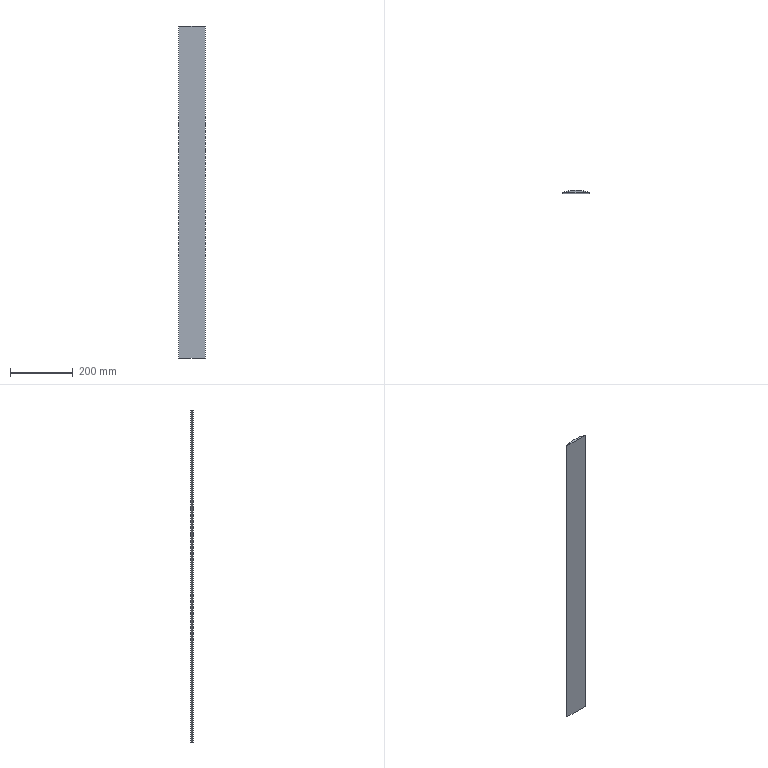Part | SolidWorks | features BaseBody 1 | 1 solid | 24 faces | box 84 x 8.038 x 1060 mm | volume 538813 mm3 | cylinder 19 | plane 5 | commonest cylinder face diameters 0.6 x8 303 x5 0.8 x4 4 x2
STEP:
#1=CARTESIAN_POINT('',(42.,-0.03816,1060.));
#2=VERTEX_POINT('',#1);
#3=CARTESIAN_POINT('',(42.,-0.03816,0.));
#4=VERTEX_POINT('',#3);
#5=CARTESIAN_POINT('',(42.,-0.03816,1060.));
#6=DIRECTION('',(0.,0.,-1.));
#7=VECTOR('',#6,1000.);
#8=LINE('',#5,#7);
#9=EDGE_CURVE('',#2,#4,#8,.T.);
#10=ORIENTED_EDGE('',*,*,#9,.F.);
#11=CARTESIAN_POINT('',(-42.,-0.03816,1060.));
#12=VERTEX_POINT('',#11);
#13=CARTESIAN_POINT('',(-40.,-0.03816,1060.));
#14=DIRECTION('',(1.,0.,0.));
#15=VECTOR('',#14,1000.);
#16=LINE('',#13,#15);
#17=EDGE_CURVE('',#12,#2,#16,.T.);
#18=ORIENTED_EDGE('',*,*,#17,.F.);
#19=CARTESIAN_POINT('',(-42.,-0.03816,0.));
#20=VERTEX_POINT('',#19);
#21=CARTESIAN_POINT('',(-42.,-0.03816,1060.));
#22=DIRECTION('',(0.,0.,1.));
#23=VECTOR('',#22,1000.);
#24=LINE('',#21,#23);
#25=EDGE_CURVE('',#20,#12,#24,.T.);
#26=ORIENTED_EDGE('',*,*,#25,.F.);
#27=CARTESIAN_POINT('',(-40.,-0.03816,0.));
#28=DIRECTION('',(-1.,0.,0.));
#29=VECTOR('',#28,1000.);
#30=LINE('',#27,#29);
#31=EDGE_CURVE('',#4,#20,#30,.T.);
#32=ORIENTED_EDGE('',*,*,#31,.F.);
#33=EDGE_LOOP('',(#10,#18,#26,#32));
#34=FACE_OUTER_BOUND('',#33,.T.);
#35=CARTESIAN_POINT('',(-40.,-0.03816,1060.));
#36=DIRECTION('',(0.,1.,0.));
#37=DIRECTION('',(-1.,0.,0.));
#38=AXIS2_PLACEMENT_3D('',#35,#36,#37);
#39=PLANE('',#38);
#40=ADVANCED_FACE('',(#34),#39,.F.);
#41=CARTESIAN_POINT('',(-40.535,2.477,0.));
#42=VERTEX_POINT('',#41);
#43=CARTESIAN_POINT('',(-42.,0.5495,0.));
#44=VERTEX_POINT('',#43);
#45=CARTESIAN_POINT('',(-40.,0.5495,0.));
#46=DIRECTION('',(0.,0.,1.));
#47=DIRECTION('',(-1.,0.,0.));
#48=AXIS2_PLACEMENT_3D('',#45,#46,#47);
#49=CIRCLE('',#48,2.);
#50=EDGE_CURVE('',#42,#44,#49,.T.);
#51=ORIENTED_EDGE('',*,*,#50,.F.);
#52=CARTESIAN_POINT('',(-25.125,5.902,0.));
#53=VERTEX_POINT('',#52);
#54=CARTESIAN_POINT('',(0.,-143.5,0.));
#55=DIRECTION('',(0.,0.,1.));
#56=DIRECTION('',(-1.,0.,0.));
#57=AXIS2_PLACEMENT_3D('',#54,#55,#56);
#58=CIRCLE('',#57,151.5);
#59=EDGE_CURVE('',#53,#42,#58,.T.);
#60=ORIENTED_EDGE('',*,*,#59,.F.);
#61=CARTESIAN_POINT('',(-24.828,5.778,0.));
#62=VERTEX_POINT('',#61);
#63=CARTESIAN_POINT('',(-25.075,5.606,0.));
#64=DIRECTION('',(0.,0.,1.));
#65=DIRECTION('',(-1.,0.,0.));
#66=AXIS2_PLACEMENT_3D('',#63,#64,#65);
#67=CIRCLE('',#66,0.3);
#68=EDGE_CURVE('',#62,#53,#67,.T.);
#69=ORIENTED_EDGE('',*,*,#68,.F.);
#70=CARTESIAN_POINT('',(-24.116,5.894,0.));
#71=VERTEX_POINT('',#70);
#72=CARTESIAN_POINT('',(-24.5,6.006,0.));
#73=DIRECTION('',(0.,0.,1.));
#74=DIRECTION('',(-1.,0.,0.));
#75=AXIS2_PLACEMENT_3D('',#72,#73,#74);
#76=CIRCLE('',#75,0.4);
#77=EDGE_CURVE('',#62,#71,#76,.T.);
#78=ORIENTED_EDGE('',*,*,#77,.T.);
#79=CARTESIAN_POINT('',(-23.875,6.107,0.));
#80=VERTEX_POINT('',#79);
#81=CARTESIAN_POINT('',(-23.828,5.811,0.));
#82=DIRECTION('',(0.,0.,1.));
#83=DIRECTION('',(-1.,0.,0.));
#84=AXIS2_PLACEMENT_3D('',#81,#82,#83);
#85=CIRCLE('',#84,0.3);
#86=EDGE_CURVE('',#80,#71,#85,.T.);
#87=ORIENTED_EDGE('',*,*,#86,.F.);
#88=CARTESIAN_POINT('',(-23.626,6.147,0.));
#89=VERTEX_POINT('',#88);
#90=CARTESIAN_POINT('',(0.,-143.5,0.));
#91=DIRECTION('',(0.,0.,1.));
#92=DIRECTION('',(-1.,0.,0.));
#93=AXIS2_PLACEMENT_3D('',#90,#91,#92);
#94=CIRCLE('',#93,151.5);
#95=EDGE_CURVE('',#89,#80,#94,.T.);
#96=ORIENTED_EDGE('',*,*,#95,.F.);
#97=CARTESIAN_POINT('',(-23.331,6.019,0.));
#98=VERTEX_POINT('',#97);
#99=CARTESIAN_POINT('',(-23.579,5.85,0.));
#100=DIRECTION('',(0.,0.,1.));
#101=DIRECTION('',(-1.,0.,0.));
#102=AXIS2_PLACEMENT_3D('',#99,#100,#101);
#103=CIRCLE('',#102,0.3);
#104=EDGE_CURVE('',#98,#89,#103,.T.);
#105=ORIENTED_EDGE('',*,*,#104,.F.);
#106=CARTESIAN_POINT('',(-22.617,6.129,0.));
#107=VERTEX_POINT('',#106);
#108=CARTESIAN_POINT('',(-23.,6.244,0.));
#109=DIRECTION('',(0.,0.,1.));
#110=DIRECTION('',(-1.,0.,0.));
#111=AXIS2_PLACEMENT_3D('',#108,#109,#110);
#112=CIRCLE('',#111,0.4);
#113=EDGE_CURVE('',#98,#107,#112,.T.);
#114=ORIENTED_EDGE('',*,*,#113,.T.);
#115=CARTESIAN_POINT('',(-22.374,6.339,0.));
#116=VERTEX_POINT('',#115);
#117=CARTESIAN_POINT('',(-22.33,6.042,0.));
#118=DIRECTION('',(0.,0.,1.));
#119=DIRECTION('',(-1.,0.,0.));
#120=AXIS2_PLACEMENT_3D('',#117,#118,#119);
#121=CIRCLE('',#120,0.3);
#122=EDGE_CURVE('',#116,#107,#121,.T.);
#123=ORIENTED_EDGE('',*,*,#122,.F.);
#124=CARTESIAN_POINT('',(22.374,6.339,0.));
#125=VERTEX_POINT('',#124);
#126=CARTESIAN_POINT('',(0.,-143.5,0.));
#127=DIRECTION('',(0.,0.,1.));
#128=DIRECTION('',(-1.,0.,0.));
#129=AXIS2_PLACEMENT_3D('',#126,#127,#128);
#130=CIRCLE('',#129,151.5);
#131=EDGE_CURVE('',#125,#116,#130,.T.);
#132=ORIENTED_EDGE('',*,*,#131,.F.);
#133=CARTESIAN_POINT('',(22.617,6.129,0.));
#134=VERTEX_POINT('',#133);
#135=CARTESIAN_POINT('',(22.33,6.042,0.));
#136=DIRECTION('',(0.,0.,1.));
#137=DIRECTION('',(-1.,0.,0.));
#138=AXIS2_PLACEMENT_3D('',#135,#136,#137);
#139=CIRCLE('',#138,0.3);
#140=EDGE_CURVE('',#134,#125,#139,.T.);
#141=ORIENTED_EDGE('',*,*,#140,.F.);
#142=CARTESIAN_POINT('',(23.331,6.019,0.));
#143=VERTEX_POINT('',#142);
#144=CARTESIAN_POINT('',(23.,6.244,0.));
#145=DIRECTION('',(0.,0.,1.));
#146=DIRECTION('',(-1.,0.,0.));
#147=AXIS2_PLACEMENT_3D('',#144,#145,#146);
#148=CIRCLE('',#147,0.4);
#149=EDGE_CURVE('',#134,#143,#148,.T.);
#150=ORIENTED_EDGE('',*,*,#149,.T.);
#151=CARTESIAN_POINT('',(23.626,6.147,0.));
#152=VERTEX_POINT('',#151);
#153=CARTESIAN_POINT('',(23.579,5.85,0.));
#154=DIRECTION('',(0.,0.,1.));
#155=DIRECTION('',(-1.,0.,0.));
#156=AXIS2_PLACEMENT_3D('',#153,#154,#155);
#157=CIRCLE('',#156,0.3);
#158=EDGE_CURVE('',#152,#143,#157,.T.);
#159=ORIENTED_EDGE('',*,*,#158,.F.);
#160=CARTESIAN_POINT('',(23.875,6.107,0.));
#161=VERTEX_POINT('',#160);
#162=CARTESIAN_POINT('',(0.,-143.5,0.));
#163=DIRECTION('',(0.,0.,1.));
#164=DIRECTION('',(-1.,0.,0.));
#165=AXIS2_PLACEMENT_3D('',#162,#163,#164);
#166=CIRCLE('',#165,151.5);
#167=EDGE_CURVE('',#161,#152,#166,.T.);
#168=ORIENTED_EDGE('',*,*,#167,.F.);
#169=CARTESIAN_POINT('',(24.116,5.894,0.));
#170=VERTEX_POINT('',#169);
#171=CARTESIAN_POINT('',(23.828,5.811,0.));
#172=DIRECTION('',(0.,0.,1.));
#173=DIRECTION('',(-1.,0.,0.));
#174=AXIS2_PLACEMENT_3D('',#171,#172,#173);
#175=CIRCLE('',#174,0.3);
#176=EDGE_CURVE('',#170,#161,#175,.T.);
#177=ORIENTED_EDGE('',*,*,#176,.F.);
#178=CARTESIAN_POINT('',(24.828,5.778,0.));
#179=VERTEX_POINT('',#178);
#180=CARTESIAN_POINT('',(24.5,6.006,0.));
#181=DIRECTION('',(0.,0.,1.));
#182=DIRECTION('',(-1.,0.,0.));
#183=AXIS2_PLACEMENT_3D('',#180,#181,#182);
#184=CIRCLE('',#183,0.4);
#185=EDGE_CURVE('',#170,#179,#184,.T.);
#186=ORIENTED_EDGE('',*,*,#185,.T.);
#187=CARTESIAN_POINT('',(25.125,5.902,0.));
#188=VERTEX_POINT('',#187);
#189=CARTESIAN_POINT('',(25.075,5.606,0.));
#190=DIRECTION('',(0.,0.,1.));
#191=DIRECTION('',(-1.,0.,0.));
#192=AXIS2_PLACEMENT_3D('',#189,#190,#191);
#193=CIRCLE('',#192,0.3);
#194=EDGE_CURVE('',#188,#179,#193,.T.);
#195=ORIENTED_EDGE('',*,*,#194,.F.);
#196=CARTESIAN_POINT('',(40.535,2.477,0.));
#197=VERTEX_POINT('',#196);
#198=CARTESIAN_POINT('',(0.,-143.5,0.));
#199=DIRECTION('',(0.,0.,1.));
#200=DIRECTION('',(-1.,0.,0.));
#201=AXIS2_PLACEMENT_3D('',#198,#199,#200);
#202=CIRCLE('',#201,151.5);
#203=EDGE_CURVE('',#197,#188,#202,.T.);
#204=ORIENTED_EDGE('',*,*,#203,.F.);
#205=CARTESIAN_POINT('',(42.,0.5495,0.));
#206=VERTEX_POINT('',#205);
#207=CARTESIAN_POINT('',(40.,0.5495,0.));
#208=DIRECTION('',(0.,0.,1.));
#209=DIRECTION('',(-1.,0.,0.));
#210=AXIS2_PLACEMENT_3D('',#207,#208,#209);
#211=CIRCLE('',#210,2.);
#212=EDGE_CURVE('',#206,#197,#211,.T.);
#213=ORIENTED_EDGE('',*,*,#212,.F.);
#214=CARTESIAN_POINT('',(42.,-143.5,0.));
#215=DIRECTION('',(0.,1.,0.));
#216=VECTOR('',#215,1000.);
#217=LINE('',#214,#216);
#218=EDGE_CURVE('',#4,#206,#217,.T.);
#219=ORIENTED_EDGE('',*,*,#218,.F.);
#220=ORIENTED_EDGE('',*,*,#31,.T.);
#221=CARTESIAN_POINT('',(-42.,-143.5,0.));
#222=DIRECTION('',(0.,-1.,0.));
#223=VECTOR('',#222,1000.);
#224=LINE('',#221,#223);
#225=EDGE_CURVE('',#44,#20,#224,.T.);
#226=ORIENTED_EDGE('',*,*,#225,.F.);
#227=EDGE_LOOP('',(#51,#60,#69,#78,#87,#96,#105,#114,#123,#132,#141,#150,#159,#168,#177,#186,#195,#204,#213,#219,#220,#226));
#228=FACE_OUTER_BOUND('',#227,.T.);
#229=CARTESIAN_POINT('',(0.,-143.5,0.));
#230=DIRECTION('',(0.,0.,1.));
#231=DIRECTION('',(1.,0.,0.));
#232=AXIS2_PLACEMENT_3D('',#229,#230,#231);
#233=PLANE('',#232);
#234=ADVANCED_FACE('',(#228),#233,.F.);
#235=CARTESIAN_POINT('',(42.,0.5495,1060.));
#236=VERTEX_POINT('',#235);
#237=CARTESIAN_POINT('',(42.,0.5495,1060.));
#238=DIRECTION('',(0.,0.,-1.));
#239=VECTOR('',#238,1000.);
#240=LINE('',#237,#239);
#241=EDGE_CURVE('',#236,#206,#240,.T.);
#242=ORIENTED_EDGE('',*,*,#241,.F.);
#243=CARTESIAN_POINT('',(42.,2.062,1060.));
#244=DIRECTION('',(0.,1.,0.));
#245=VECTOR('',#244,1000.);
#246=LINE('',#243,#245);
#247=EDGE_CURVE('',#2,#236,#246,.T.);
#248=ORIENTED_EDGE('',*,*,#247,.F.);
#249=ORIENTED_EDGE('',*,*,#9,.T.);
#250=ORIENTED_EDGE('',*,*,#218,.T.);
#251=EDGE_LOOP('',(#242,#248,#249,#250));
#252=FACE_OUTER_BOUND('',#251,.T.);
#253=CARTESIAN_POINT('',(42.,2.062,1060.));
#254=DIRECTION('',(-1.,0.,0.));
#255=DIRECTION('',(0.,0.,1.));
#256=AXIS2_PLACEMENT_3D('',#253,#254,#255);
#257=PLANE('',#256);
#258=ADVANCED_FACE('',(#252),#257,.F.);
#259=CARTESIAN_POINT('',(-24.116,5.894,1060.));
#260=VERTEX_POINT('',#259);
#261=CARTESIAN_POINT('',(-24.828,5.778,1060.));
#262=VERTEX_POINT('',#261);
#263=CARTESIAN_POINT('',(-24.5,6.006,1060.));
#264=DIRECTION('',(0.,0.,-1.));
#265=DIRECTION('',(-1.,0.,0.));
#266=AXIS2_PLACEMENT_3D('',#263,#264,#265);
#267=CIRCLE('',#266,0.4);
#268=EDGE_CURVE('',#260,#262,#267,.T.);
#269=ORIENTED_EDGE('',*,*,#268,.T.);
#270=CARTESIAN_POINT('',(-25.125,5.902,1060.));
#271=VERTEX_POINT('',#270);
#272=CARTESIAN_POINT('',(-25.075,5.606,1060.));
#273=DIRECTION('',(0.,0.,-1.));
#274=DIRECTION('',(-1.,0.,0.));
#275=AXIS2_PLACEMENT_3D('',#272,#273,#274);
#276=CIRCLE('',#275,0.3);
#277=EDGE_CURVE('',#271,#262,#276,.T.);
#278=ORIENTED_EDGE('',*,*,#277,.F.);
#279=CARTESIAN_POINT('',(-40.535,2.477,1060.));
#280=VERTEX_POINT('',#279);
#281=CARTESIAN_POINT('',(0.,-143.5,1060.));
#282=DIRECTION('',(0.,0.,1.));
#283=DIRECTION('',(-1.,0.,0.));
#284=AXIS2_PLACEMENT_3D('',#281,#282,#283);
#285=CIRCLE('',#284,151.5);
#286=EDGE_CURVE('',#271,#280,#285,.T.);
#287=ORIENTED_EDGE('',*,*,#286,.T.);
#288=CARTESIAN_POINT('',(-42.,0.5495,1060.));
#289=VERTEX_POINT('',#288);
#290=CARTESIAN_POINT('',(-40.,0.5495,1060.));
#291=DIRECTION('',(0.,0.,1.));
#292=DIRECTION('',(-1.,0.,0.));
#293=AXIS2_PLACEMENT_3D('',#290,#291,#292);
#294=CIRCLE('',#293,2.);
#295=EDGE_CURVE('',#280,#289,#294,.T.);
#296=ORIENTED_EDGE('',*,*,#295,.T.);
#297=CARTESIAN_POINT('',(-42.,-143.5,1060.));
#298=DIRECTION('',(0.,-1.,0.));
#299=VECTOR('',#298,1000.);
#300=LINE('',#297,#299);
#301=EDGE_CURVE('',#289,#12,#300,.T.);
#302=ORIENTED_EDGE('',*,*,#301,.T.);
#303=ORIENTED_EDGE('',*,*,#17,.T.);
#304=ORIENTED_EDGE('',*,*,#247,.T.);
#305=CARTESIAN_POINT('',(40.535,2.477,1060.));
#306=VERTEX_POINT('',#305);
#307=CARTESIAN_POINT('',(40.,0.5495,1060.));
#308=DIRECTION('',(0.,0.,1.));
#309=DIRECTION('',(-1.,0.,0.));
#310=AXIS2_PLACEMENT_3D('',#307,#308,#309);
#311=CIRCLE('',#310,2.);
#312=EDGE_CURVE('',#236,#306,#311,.T.);
#313=ORIENTED_EDGE('',*,*,#312,.T.);
#314=CARTESIAN_POINT('',(25.125,5.902,1060.));
#315=VERTEX_POINT('',#314);
#316=CARTESIAN_POINT('',(0.,-143.5,1060.));
#317=DIRECTION('',(0.,0.,1.));
#318=DIRECTION('',(-1.,0.,0.));
#319=AXIS2_PLACEMENT_3D('',#316,#317,#318);
#320=CIRCLE('',#319,151.5);
#321=EDGE_CURVE('',#306,#315,#320,.T.);
#322=ORIENTED_EDGE('',*,*,#321,.T.);
#323=CARTESIAN_POINT('',(24.828,5.778,1060.));
#324=VERTEX_POINT('',#323);
#325=CARTESIAN_POINT('',(25.075,5.606,1060.));
#326=DIRECTION('',(0.,0.,-1.));
#327=DIRECTION('',(-1.,0.,0.));
#328=AXIS2_PLACEMENT_3D('',#325,#326,#327);
#329=CIRCLE('',#328,0.3);
#330=EDGE_CURVE('',#324,#315,#329,.T.);
#331=ORIENTED_EDGE('',*,*,#330,.F.);
#332=CARTESIAN_POINT('',(24.116,5.894,1060.));
#333=VERTEX_POINT('',#332);
#334=CARTESIAN_POINT('',(24.5,6.006,1060.));
#335=DIRECTION('',(0.,0.,-1.));
#336=DIRECTION('',(-1.,0.,0.));
#337=AXIS2_PLACEMENT_3D('',#334,#335,#336);
#338=CIRCLE('',#337,0.4);
#339=EDGE_CURVE('',#324,#333,#338,.T.);
#340=ORIENTED_EDGE('',*,*,#339,.T.);
#341=CARTESIAN_POINT('',(23.875,6.107,1060.));
#342=VERTEX_POINT('',#341);
#343=CARTESIAN_POINT('',(23.828,5.811,1060.));
#344=DIRECTION('',(0.,0.,-1.));
#345=DIRECTION('',(-1.,0.,0.));
#346=AXIS2_PLACEMENT_3D('',#343,#344,#345);
#347=CIRCLE('',#346,0.3);
#348=EDGE_CURVE('',#342,#333,#347,.T.);
#349=ORIENTED_EDGE('',*,*,#348,.F.);
#350=CARTESIAN_POINT('',(23.626,6.147,1060.));
#351=VERTEX_POINT('',#350);
#352=CARTESIAN_POINT('',(0.,-143.5,1060.));
#353=DIRECTION('',(0.,0.,-1.));
#354=DIRECTION('',(-1.,0.,0.));
#355=AXIS2_PLACEMENT_3D('',#352,#353,#354);
#356=CIRCLE('',#355,151.5);
#357=EDGE_CURVE('',#351,#342,#356,.T.);
#358=ORIENTED_EDGE('',*,*,#357,.F.);
#359=CARTESIAN_POINT('',(23.331,6.019,1060.));
#360=VERTEX_POINT('',#359);
#361=CARTESIAN_POINT('',(23.579,5.85,1060.));
#362=DIRECTION('',(0.,0.,-1.));
#363=DIRECTION('',(-1.,0.,0.));
#364=AXIS2_PLACEMENT_3D('',#361,#362,#363);
#365=CIRCLE('',#364,0.3);
#366=EDGE_CURVE('',#360,#351,#365,.T.);
#367=ORIENTED_EDGE('',*,*,#366,.F.);
#368=CARTESIAN_POINT('',(22.617,6.129,1060.));
#369=VERTEX_POINT('',#368);
#370=CARTESIAN_POINT('',(23.,6.244,1060.));
#371=DIRECTION('',(0.,0.,-1.));
#372=DIRECTION('',(-1.,0.,0.));
#373=AXIS2_PLACEMENT_3D('',#370,#371,#372);
#374=CIRCLE('',#373,0.4);
#375=EDGE_CURVE('',#360,#369,#374,.T.);
#376=ORIENTED_EDGE('',*,*,#375,.T.);
#377=CARTESIAN_POINT('',(22.374,6.339,1060.));
#378=VERTEX_POINT('',#377);
#379=CARTESIAN_POINT('',(22.33,6.042,1060.));
#380=DIRECTION('',(0.,0.,-1.));
#381=DIRECTION('',(-1.,0.,0.));
#382=AXIS2_PLACEMENT_3D('',#379,#380,#381);
#383=CIRCLE('',#382,0.3);
#384=EDGE_CURVE('',#378,#369,#383,.T.);
#385=ORIENTED_EDGE('',*,*,#384,.F.);
#386=CARTESIAN_POINT('',(-22.374,6.339,1060.));
#387=VERTEX_POINT('',#386);
#388=CARTESIAN_POINT('',(0.,-143.5,1060.));
#389=DIRECTION('',(0.,0.,1.));
#390=DIRECTION('',(-1.,0.,0.));
#391=AXIS2_PLACEMENT_3D('',#388,#389,#390);
#392=CIRCLE('',#391,151.5);
#393=EDGE_CURVE('',#378,#387,#392,.T.);
#394=ORIENTED_EDGE('',*,*,#393,.T.);
#395=CARTESIAN_POINT('',(-22.617,6.129,1060.));
#396=VERTEX_POINT('',#395);
#397=CARTESIAN_POINT('',(-22.33,6.042,1060.));
#398=DIRECTION('',(0.,0.,-1.));
#399=DIRECTION('',(-1.,0.,0.));
#400=AXIS2_PLACEMENT_3D('',#397,#398,#399);
#401=CIRCLE('',#400,0.3);
#402=EDGE_CURVE('',#396,#387,#401,.T.);
#403=ORIENTED_EDGE('',*,*,#402,.F.);
#404=CARTESIAN_POINT('',(-23.331,6.019,1060.));
#405=VERTEX_POINT('',#404);
#406=CARTESIAN_POINT('',(-23.,6.244,1060.));
#407=DIRECTION('',(0.,0.,-1.));
#408=DIRECTION('',(-1.,0.,0.));
#409=AXIS2_PLACEMENT_3D('',#406,#407,#408);
#410=CIRCLE('',#409,0.4);
#411=EDGE_CURVE('',#396,#405,#410,.T.);
#412=ORIENTED_EDGE('',*,*,#411,.T.);
#413=CARTESIAN_POINT('',(-23.626,6.147,1060.));
#414=VERTEX_POINT('',#413);
#415=CARTESIAN_POINT('',(-23.579,5.85,1060.));
#416=DIRECTION('',(0.,0.,-1.));
#417=DIRECTION('',(-1.,0.,0.));
#418=AXIS2_PLACEMENT_3D('',#415,#416,#417);
#419=CIRCLE('',#418,0.3);
#420=EDGE_CURVE('',#414,#405,#419,.T.);
#421=ORIENTED_EDGE('',*,*,#420,.F.);
#422=CARTESIAN_POINT('',(-23.875,6.107,1060.));
#423=VERTEX_POINT('',#422);
#424=CARTESIAN_POINT('',(0.,-143.5,1060.));
#425=DIRECTION('',(0.,0.,-1.));
#426=DIRECTION('',(-1.,0.,0.));
#427=AXIS2_PLACEMENT_3D('',#424,#425,#426);
#428=CIRCLE('',#427,151.5);
#429=EDGE_CURVE('',#423,#414,#428,.T.);
#430=ORIENTED_EDGE('',*,*,#429,.F.);
#431=CARTESIAN_POINT('',(-23.828,5.811,1060.));
#432=DIRECTION('',(0.,0.,-1.));
#433=DIRECTION('',(-1.,0.,0.));
#434=AXIS2_PLACEMENT_3D('',#431,#432,#433);
#435=CIRCLE('',#434,0.3);
#436=EDGE_CURVE('',#260,#423,#435,.T.);
#437=ORIENTED_EDGE('',*,*,#436,.F.);
#438=EDGE_LOOP('',(#269,#278,#287,#296,#302,#303,#304,#313,#322,#331,#340,#349,#358,#367,#376,#385,#394,#403,#412,#421,#430,#437));
#439=FACE_OUTER_BOUND('',#438,.T.);
#440=CARTESIAN_POINT('',(0.,-143.5,1060.));
#441=DIRECTION('',(0.,0.,1.));
#442=DIRECTION('',(1.,0.,0.));
#443=AXIS2_PLACEMENT_3D('',#440,#441,#442);
#444=PLANE('',#443);
#445=ADVANCED_FACE('',(#439),#444,.T.);
#446=CARTESIAN_POINT('',(-42.,0.5495,1060.));
#447=DIRECTION('',(0.,0.,1.));
#448=VECTOR('',#447,1000.);
#449=LINE('',#446,#448);
#450=EDGE_CURVE('',#44,#289,#449,.T.);
#451=ORIENTED_EDGE('',*,*,#450,.F.);
#452=ORIENTED_EDGE('',*,*,#225,.T.);
#453=ORIENTED_EDGE('',*,*,#25,.T.);
#454=ORIENTED_EDGE('',*,*,#301,.F.);
#455=EDGE_LOOP('',(#451,#452,#453,#454));
#456=FACE_OUTER_BOUND('',#455,.T.);
#457=CARTESIAN_POINT('',(-42.,2.062,1060.));
#458=DIRECTION('',(1.,0.,0.));
#459=DIRECTION('',(0.,0.,-1.));
#460=AXIS2_PLACEMENT_3D('',#457,#458,#459);
#461=PLANE('',#460);
#462=ADVANCED_FACE('',(#456),#461,.F.);
#463=ORIENTED_EDGE('',*,*,#50,.T.);
#464=ORIENTED_EDGE('',*,*,#450,.T.);
#465=ORIENTED_EDGE('',*,*,#295,.F.);
#466=CARTESIAN_POINT('',(-40.535,2.477,1060.));
#467=DIRECTION('',(0.,0.,-1.));
#468=VECTOR('',#467,1000.);
#469=LINE('',#466,#468);
#470=EDGE_CURVE('',#280,#42,#469,.T.);
#471=ORIENTED_EDGE('',*,*,#470,.T.);
#472=EDGE_LOOP('',(#463,#464,#465,#471));
#473=FACE_OUTER_BOUND('',#472,.T.);
#474=CARTESIAN_POINT('',(-40.,0.5495,1060.));
#475=DIRECTION('',(0.,0.,-1.));
#476=DIRECTION('',(-1.,0.,0.));
#477=AXIS2_PLACEMENT_3D('',#474,#475,#476);
#478=CYLINDRICAL_SURFACE('',#477,2.);
#479=ADVANCED_FACE('',(#473),#478,.T.);
#480=ORIENTED_EDGE('',*,*,#286,.F.);
#481=CARTESIAN_POINT('',(-25.125,5.902,1060.));
#482=DIRECTION('',(0.,0.,-1.));
#483=VECTOR('',#482,1000.);
#484=LINE('',#481,#483);
#485=EDGE_CURVE('',#271,#53,#484,.T.);
#486=ORIENTED_EDGE('',*,*,#485,.T.);
#487=ORIENTED_EDGE('',*,*,#59,.T.);
#488=ORIENTED_EDGE('',*,*,#470,.F.);
#489=EDGE_LOOP('',(#480,#486,#487,#488));
#490=FACE_OUTER_BOUND('',#489,.T.);
#491=CARTESIAN_POINT('',(0.,-143.5,1060.));
#492=DIRECTION('',(0.,0.,-1.));
#493=DIRECTION('',(-1.,0.,0.));
#494=AXIS2_PLACEMENT_3D('',#491,#492,#493);
#495=CYLINDRICAL_SURFACE('',#494,151.5);
#496=ADVANCED_FACE('',(#490),#495,.T.);
#497=ORIENTED_EDGE('',*,*,#393,.F.);
#498=CARTESIAN_POINT('',(22.374,6.339,1060.));
#499=DIRECTION('',(0.,0.,-1.));
#500=VECTOR('',#499,1000.);
#501=LINE('',#498,#500);
#502=EDGE_CURVE('',#378,#125,#501,.T.);
#503=ORIENTED_EDGE('',*,*,#502,.T.);
#504=ORIENTED_EDGE('',*,*,#131,.T.);
#505=CARTESIAN_POINT('',(-22.374,6.339,1060.));
#506=DIRECTION('',(0.,0.,1.));
#507=VECTOR('',#506,1000.);
#508=LINE('',#505,#507);
#509=EDGE_CURVE('',#116,#387,#508,.T.);
#510=ORIENTED_EDGE('',*,*,#509,.T.);
#511=EDGE_LOOP('',(#497,#503,#504,#510));
#512=FACE_OUTER_BOUND('',#511,.T.);
#513=CARTESIAN_POINT('',(0.,-143.5,1060.));
#514=DIRECTION('',(0.,0.,-1.));
#515=DIRECTION('',(-1.,0.,0.));
#516=AXIS2_PLACEMENT_3D('',#513,#514,#515);
#517=CYLINDRICAL_SURFACE('',#516,151.5);
#518=ADVANCED_FACE('',(#512),#517,.T.);
#519=ORIENTED_EDGE('',*,*,#203,.T.);
#520=CARTESIAN_POINT('',(25.125,5.902,1060.));
#521=DIRECTION('',(0.,0.,1.));
#522=VECTOR('',#521,1000.);
#523=LINE('',#520,#522);
#524=EDGE_CURVE('',#188,#315,#523,.T.);
#525=ORIENTED_EDGE('',*,*,#524,.T.);
#526=ORIENTED_EDGE('',*,*,#321,.F.);
#527=CARTESIAN_POINT('',(40.535,2.477,1060.));
#528=DIRECTION('',(0.,0.,-1.));
#529=VECTOR('',#528,1000.);
#530=LINE('',#527,#529);
#531=EDGE_CURVE('',#306,#197,#530,.T.);
#532=ORIENTED_EDGE('',*,*,#531,.T.);
#533=EDGE_LOOP('',(#519,#525,#526,#532));
#534=FACE_OUTER_BOUND('',#533,.T.);
#535=CARTESIAN_POINT('',(0.,-143.5,1060.));
#536=DIRECTION('',(0.,0.,-1.));
#537=DIRECTION('',(-1.,0.,0.));
#538=AXIS2_PLACEMENT_3D('',#535,#536,#537);
#539=CYLINDRICAL_SURFACE('',#538,151.5);
#540=ADVANCED_FACE('',(#534),#539,.T.);
#541=ORIENTED_EDGE('',*,*,#212,.T.);
#542=ORIENTED_EDGE('',*,*,#531,.F.);
#543=ORIENTED_EDGE('',*,*,#312,.F.);
#544=ORIENTED_EDGE('',*,*,#241,.T.);
#545=EDGE_LOOP('',(#541,#542,#543,#544));
#546=FACE_OUTER_BOUND('',#545,.T.);
#547=CARTESIAN_POINT('',(40.,0.5495,1060.));
#548=DIRECTION('',(0.,0.,-1.));
#549=DIRECTION('',(-1.,0.,0.));
#550=AXIS2_PLACEMENT_3D('',#547,#548,#549);
#551=CYLINDRICAL_SURFACE('',#550,2.);
#552=ADVANCED_FACE('',(#546),#551,.T.);
#553=ORIENTED_EDGE('',*,*,#277,.T.);
#554=CARTESIAN_POINT('',(-24.828,5.778,1060.));
#555=DIRECTION('',(0.,0.,-1.));
#556=VECTOR('',#555,1000.);
#557=LINE('',#554,#556);
#558=EDGE_CURVE('',#262,#62,#557,.T.);
#559=ORIENTED_EDGE('',*,*,#558,.T.);
#560=ORIENTED_EDGE('',*,*,#68,.T.);
#561=ORIENTED_EDGE('',*,*,#485,.F.);
#562=EDGE_LOOP('',(#553,#559,#560,#561));
#563=FACE_OUTER_BOUND('',#562,.T.);
#564=CARTESIAN_POINT('',(-25.075,5.606,1060.));
#565=DIRECTION('',(0.,0.,-1.));
#566=DIRECTION('',(-1.,0.,0.));
#567=AXIS2_PLACEMENT_3D('',#564,#565,#566);
#568=CYLINDRICAL_SURFACE('',#567,0.3);
#569=ADVANCED_FACE('',(#563),#568,.T.);
#570=ORIENTED_EDGE('',*,*,#384,.T.);
#571=CARTESIAN_POINT('',(22.617,6.129,1060.));
#572=DIRECTION('',(0.,0.,-1.));
#573=VECTOR('',#572,1000.);
#574=LINE('',#571,#573);
#575=EDGE_CURVE('',#369,#134,#574,.T.);
#576=ORIENTED_EDGE('',*,*,#575,.T.);
#577=ORIENTED_EDGE('',*,*,#140,.T.);
#578=ORIENTED_EDGE('',*,*,#502,.F.);
#579=EDGE_LOOP('',(#570,#576,#577,#578));
#580=FACE_OUTER_BOUND('',#579,.T.);
#581=CARTESIAN_POINT('',(22.33,6.042,1060.));
#582=DIRECTION('',(0.,0.,-1.));
#583=DIRECTION('',(-1.,0.,0.));
#584=AXIS2_PLACEMENT_3D('',#581,#582,#583);
#585=CYLINDRICAL_SURFACE('',#584,0.3);
#586=ADVANCED_FACE('',(#580),#585,.T.);
#587=ORIENTED_EDGE('',*,*,#402,.T.);
#588=ORIENTED_EDGE('',*,*,#509,.F.);
#589=ORIENTED_EDGE('',*,*,#122,.T.);
#590=CARTESIAN_POINT('',(-22.617,6.129,1060.));
#591=DIRECTION('',(0.,0.,1.));
#592=VECTOR('',#591,1000.);
#593=LINE('',#590,#592);
#594=EDGE_CURVE('',#107,#396,#593,.T.);
#595=ORIENTED_EDGE('',*,*,#594,.T.);
#596=EDGE_LOOP('',(#587,#588,#589,#595));
#597=FACE_OUTER_BOUND('',#596,.T.);
#598=CARTESIAN_POINT('',(-22.33,6.042,1060.));
#599=DIRECTION('',(0.,0.,-1.));
#600=DIRECTION('',(-1.,0.,0.));
#601=AXIS2_PLACEMENT_3D('',#598,#599,#600);
#602=CYLINDRICAL_SURFACE('',#601,0.3);
#603=ADVANCED_FACE('',(#597),#602,.T.);
#604=ORIENTED_EDGE('',*,*,#330,.T.);
#605=ORIENTED_EDGE('',*,*,#524,.F.);
#606=ORIENTED_EDGE('',*,*,#194,.T.);
#607=CARTESIAN_POINT('',(24.828,5.778,1060.));
#608=DIRECTION('',(0.,0.,1.));
#609=VECTOR('',#608,1000.);
#610=LINE('',#607,#609);
#611=EDGE_CURVE('',#179,#324,#610,.T.);
#612=ORIENTED_EDGE('',*,*,#611,.T.);
#613=EDGE_LOOP('',(#604,#605,#606,#612));
#614=FACE_OUTER_BOUND('',#613,.T.);
#615=CARTESIAN_POINT('',(25.075,5.606,1060.));
#616=DIRECTION('',(0.,0.,-1.));
#617=DIRECTION('',(-1.,0.,0.));
#618=AXIS2_PLACEMENT_3D('',#615,#616,#617);
#619=CYLINDRICAL_SURFACE('',#618,0.3);
#620=ADVANCED_FACE('',(#614),#619,.T.);
#621=ORIENTED_EDGE('',*,*,#558,.F.);
#622=ORIENTED_EDGE('',*,*,#268,.F.);
#623=CARTESIAN_POINT('',(-24.116,5.894,1060.));
#624=DIRECTION('',(0.,0.,1.));
#625=VECTOR('',#624,1000.);
#626=LINE('',#623,#625);
#627=EDGE_CURVE('',#71,#260,#626,.T.);
#628=ORIENTED_EDGE('',*,*,#627,.F.);
#629=ORIENTED_EDGE('',*,*,#77,.F.);
#630=EDGE_LOOP('',(#621,#622,#628,#629));
#631=FACE_OUTER_BOUND('',#630,.T.);
#632=CARTESIAN_POINT('',(-24.5,6.006,1060.));
#633=DIRECTION('',(0.,0.,-1.));
#634=DIRECTION('',(-1.,0.,0.));
#635=AXIS2_PLACEMENT_3D('',#632,#633,#634);
#636=CYLINDRICAL_SURFACE('',#635,0.4);
#637=ADVANCED_FACE('',(#631),#636,.F.);
#638=ORIENTED_EDGE('',*,*,#575,.F.);
#639=ORIENTED_EDGE('',*,*,#375,.F.);
#640=CARTESIAN_POINT('',(23.331,6.019,1060.));
#641=DIRECTION('',(0.,0.,1.));
#642=VECTOR('',#641,1000.);
#643=LINE('',#640,#642);
#644=EDGE_CURVE('',#143,#360,#643,.T.);
#645=ORIENTED_EDGE('',*,*,#644,.F.);
#646=ORIENTED_EDGE('',*,*,#149,.F.);
#647=EDGE_LOOP('',(#638,#639,#645,#646));
#648=FACE_OUTER_BOUND('',#647,.T.);
#649=CARTESIAN_POINT('',(23.,6.244,1060.));
#650=DIRECTION('',(0.,0.,-1.));
#651=DIRECTION('',(-1.,0.,0.));
#652=AXIS2_PLACEMENT_3D('',#649,#650,#651);
#653=CYLINDRICAL_SURFACE('',#652,0.4);
#654=ADVANCED_FACE('',(#648),#653,.F.);
#655=CARTESIAN_POINT('',(-23.331,6.019,1060.));
#656=DIRECTION('',(0.,0.,-1.));
#657=VECTOR('',#656,1000.);
#658=LINE('',#655,#657);
#659=EDGE_CURVE('',#405,#98,#658,.T.);
#660=ORIENTED_EDGE('',*,*,#659,.F.);
#661=ORIENTED_EDGE('',*,*,#411,.F.);
#662=ORIENTED_EDGE('',*,*,#594,.F.);
#663=ORIENTED_EDGE('',*,*,#113,.F.);
#664=EDGE_LOOP('',(#660,#661,#662,#663));
#665=FACE_OUTER_BOUND('',#664,.T.);
#666=CARTESIAN_POINT('',(-23.,6.244,1060.));
#667=DIRECTION('',(0.,0.,-1.));
#668=DIRECTION('',(-1.,0.,0.));
#669=AXIS2_PLACEMENT_3D('',#666,#667,#668);
#670=CYLINDRICAL_SURFACE('',#669,0.4);
#671=ADVANCED_FACE('',(#665),#670,.F.);
#672=CARTESIAN_POINT('',(24.116,5.894,1060.));
#673=DIRECTION('',(0.,0.,-1.));
#674=VECTOR('',#673,1000.);
#675=LINE('',#672,#674);
#676=EDGE_CURVE('',#333,#170,#675,.T.);
#677=ORIENTED_EDGE('',*,*,#676,.F.);
#678=ORIENTED_EDGE('',*,*,#339,.F.);
#679=ORIENTED_EDGE('',*,*,#611,.F.);
#680=ORIENTED_EDGE('',*,*,#185,.F.);
#681=EDGE_LOOP('',(#677,#678,#679,#680));
#682=FACE_OUTER_BOUND('',#681,.T.);
#683=CARTESIAN_POINT('',(24.5,6.006,1060.));
#684=DIRECTION('',(0.,0.,-1.));
#685=DIRECTION('',(-1.,0.,0.));
#686=AXIS2_PLACEMENT_3D('',#683,#684,#685);
#687=CYLINDRICAL_SURFACE('',#686,0.4);
#688=ADVANCED_FACE('',(#682),#687,.F.);
#689=ORIENTED_EDGE('',*,*,#436,.T.);
#690=CARTESIAN_POINT('',(-23.875,6.107,1060.));
#691=DIRECTION('',(0.,0.,-1.));
#692=VECTOR('',#691,1000.);
#693=LINE('',#690,#692);
#694=EDGE_CURVE('',#423,#80,#693,.T.);
#695=ORIENTED_EDGE('',*,*,#694,.T.);
#696=ORIENTED_EDGE('',*,*,#86,.T.);
#697=ORIENTED_EDGE('',*,*,#627,.T.);
#698=EDGE_LOOP('',(#689,#695,#696,#697));
#699=FACE_OUTER_BOUND('',#698,.T.);
#700=CARTESIAN_POINT('',(-23.828,5.811,1060.));
#701=DIRECTION('',(0.,0.,-1.));
#702=DIRECTION('',(-1.,0.,0.));
#703=AXIS2_PLACEMENT_3D('',#700,#701,#702);
#704=CYLINDRICAL_SURFACE('',#703,0.3);
#705=ADVANCED_FACE('',(#699),#704,.T.);
#706=ORIENTED_EDGE('',*,*,#366,.T.);
#707=CARTESIAN_POINT('',(23.626,6.147,1060.));
#708=DIRECTION('',(0.,0.,-1.));
#709=VECTOR('',#708,1000.);
#710=LINE('',#707,#709);
#711=EDGE_CURVE('',#351,#152,#710,.T.);
#712=ORIENTED_EDGE('',*,*,#711,.T.);
#713=ORIENTED_EDGE('',*,*,#158,.T.);
#714=ORIENTED_EDGE('',*,*,#644,.T.);
#715=EDGE_LOOP('',(#706,#712,#713,#714));
#716=FACE_OUTER_BOUND('',#715,.T.);
#717=CARTESIAN_POINT('',(23.579,5.85,1060.));
#718=DIRECTION('',(0.,0.,-1.));
#719=DIRECTION('',(-1.,0.,0.));
#720=AXIS2_PLACEMENT_3D('',#717,#718,#719);
#721=CYLINDRICAL_SURFACE('',#720,0.3);
#722=ADVANCED_FACE('',(#716),#721,.T.);
#723=ORIENTED_EDGE('',*,*,#420,.T.);
#724=ORIENTED_EDGE('',*,*,#659,.T.);
#725=ORIENTED_EDGE('',*,*,#104,.T.);
#726=CARTESIAN_POINT('',(-23.626,6.147,1060.));
#727=DIRECTION('',(0.,0.,1.));
#728=VECTOR('',#727,1000.);
#729=LINE('',#726,#728);
#730=EDGE_CURVE('',#89,#414,#729,.T.);
#731=ORIENTED_EDGE('',*,*,#730,.T.);
#732=EDGE_LOOP('',(#723,#724,#725,#731));
#733=FACE_OUTER_BOUND('',#732,.T.);
#734=CARTESIAN_POINT('',(-23.579,5.85,1060.));
#735=DIRECTION('',(0.,0.,-1.));
#736=DIRECTION('',(-1.,0.,0.));
#737=AXIS2_PLACEMENT_3D('',#734,#735,#736);
#738=CYLINDRICAL_SURFACE('',#737,0.3);
#739=ADVANCED_FACE('',(#733),#738,.T.);
#740=ORIENTED_EDGE('',*,*,#348,.T.);
#741=ORIENTED_EDGE('',*,*,#676,.T.);
#742=ORIENTED_EDGE('',*,*,#176,.T.);
#743=CARTESIAN_POINT('',(23.875,6.107,1060.));
#744=DIRECTION('',(0.,0.,1.));
#745=VECTOR('',#744,1000.);
#746=LINE('',#743,#745);
#747=EDGE_CURVE('',#161,#342,#746,.T.);
#748=ORIENTED_EDGE('',*,*,#747,.T.);
#749=EDGE_LOOP('',(#740,#741,#742,#748));
#750=FACE_OUTER_BOUND('',#749,.T.);
#751=CARTESIAN_POINT('',(23.828,5.811,1060.));
#752=DIRECTION('',(0.,0.,-1.));
#753=DIRECTION('',(-1.,0.,0.));
#754=AXIS2_PLACEMENT_3D('',#751,#752,#753);
#755=CYLINDRICAL_SURFACE('',#754,0.3);
#756=ADVANCED_FACE('',(#750),#755,.T.);
#757=ORIENTED_EDGE('',*,*,#429,.T.);
#758=ORIENTED_EDGE('',*,*,#730,.F.);
#759=ORIENTED_EDGE('',*,*,#95,.T.);
#760=ORIENTED_EDGE('',*,*,#694,.F.);
#761=EDGE_LOOP('',(#757,#758,#759,#760));
#762=FACE_OUTER_BOUND('',#761,.T.);
#763=CARTESIAN_POINT('',(0.,-143.5,1060.));
#764=DIRECTION('',(0.,0.,-1.));
#765=DIRECTION('',(-1.,0.,0.));
#766=AXIS2_PLACEMENT_3D('',#763,#764,#765);
#767=CYLINDRICAL_SURFACE('',#766,151.5);
#768=ADVANCED_FACE('',(#762),#767,.T.);
#769=ORIENTED_EDGE('',*,*,#357,.T.);
#770=ORIENTED_EDGE('',*,*,#747,.F.);
#771=ORIENTED_EDGE('',*,*,#167,.T.);
#772=ORIENTED_EDGE('',*,*,#711,.F.);
#773=EDGE_LOOP('',(#769,#770,#771,#772));
#774=FACE_OUTER_BOUND('',#773,.T.);
#775=CARTESIAN_POINT('',(0.,-143.5,1060.));
#776=DIRECTION('',(0.,0.,-1.));
#777=DIRECTION('',(-1.,0.,0.));
#778=AXIS2_PLACEMENT_3D('',#775,#776,#777);
#779=CYLINDRICAL_SURFACE('',#778,151.5);
#780=ADVANCED_FACE('',(#774),#779,.T.);
#781=CLOSED_SHELL('',(#40,#234,#258,#445,#462,#479,#496,#518,#540,#552,#569,#586,#603,#620,#637,#654,#671,#688,#705,#722,#739,#756,#768,#780));
#782=MANIFOLD_SOLID_BREP('',#781);
#783=CARTESIAN_POINT('',(0.,0.,0.));
#784=DIRECTION('',(0.,0.,1.));
#785=DIRECTION('',(1.,0.,0.));
#786=AXIS2_PLACEMENT_3D('',#783,#784,#785);
#787=(LENGTH_UNIT()NAMED_UNIT(*)SI_UNIT(.MILLI.,.METRE.));
#788=UNCERTAINTY_MEASURE_WITH_UNIT(LENGTH_MEASURE(0.00001),#787,'','');
#789=(NAMED_UNIT(*)PLANE_ANGLE_UNIT()SI_UNIT($,.RADIAN.));
#790=(NAMED_UNIT(*)SI_UNIT($,.STERADIAN.)SOLID_ANGLE_UNIT());
#791=(GEOMETRIC_REPRESENTATION_CONTEXT(3)GLOBAL_UNCERTAINTY_ASSIGNED_CONTEXT((#788))GLOBAL_UNIT_ASSIGNED_CONTEXT((#787,#789,#790))REPRESENTATION_CONTEXT('',''));
#792=ADVANCED_BREP_SHAPE_REPRESENTATION('',(#782,#786),#791);